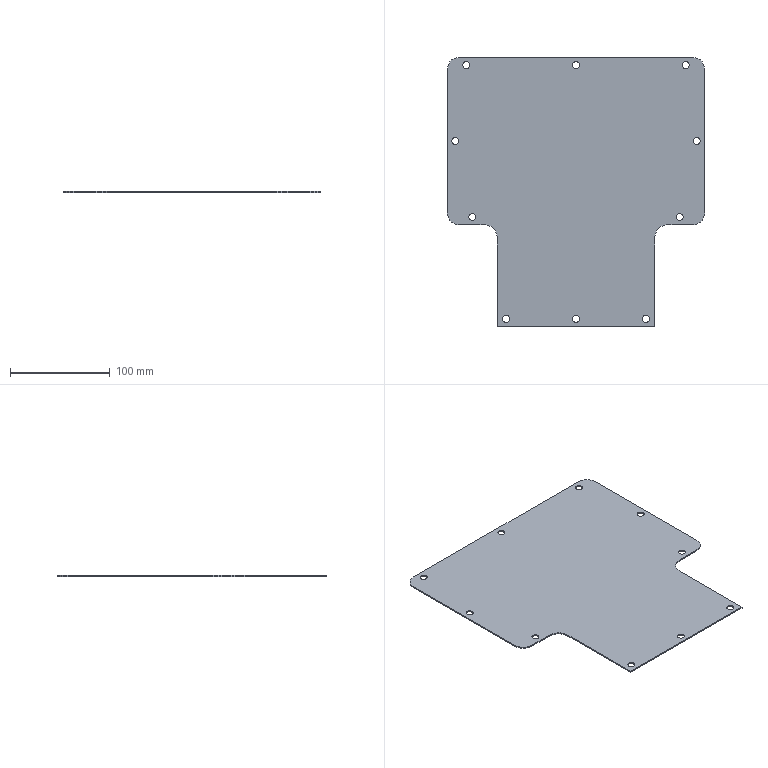Part | SolidWorks | features FlatPattern 1, SMBaseFlange 1, SheetMetal 1 | 1 solid | 36 faces | box 257.6 x 269.6 x 1.2 mm | volume 70578 mm3 | cylinder 26 | plane 10 | commonest cylinder face diameters 7 x20 24 x4 26.4 x2
STEP:
#1=CARTESIAN_POINT('',(14.652,27.28,-1.2));
#2=VERTEX_POINT('',#1);
#3=CARTESIAN_POINT('',(7.652,27.28,-1.2));
#4=VERTEX_POINT('',#3);
#5=CARTESIAN_POINT('',(11.152,27.28,-1.2));
#6=DIRECTION('',(0.,0.,-1.));
#7=DIRECTION('',(-1.,0.,0.));
#8=AXIS2_PLACEMENT_3D('',#5,#6,#7);
#9=CIRCLE('',#8,3.5);
#10=EDGE_CURVE('',#2,#4,#9,.T.);
#11=ORIENTED_EDGE('',*,*,#10,.T.);
#12=CARTESIAN_POINT('',(7.652,27.28,0.));
#13=VERTEX_POINT('',#12);
#14=CARTESIAN_POINT('',(7.652,27.28,-1.2));
#15=DIRECTION('',(0.,0.,1.));
#16=VECTOR('',#15,1000.);
#17=LINE('',#14,#16);
#18=EDGE_CURVE('',#4,#13,#17,.T.);
#19=ORIENTED_EDGE('',*,*,#18,.T.);
#20=CARTESIAN_POINT('',(14.652,27.28,0.));
#21=VERTEX_POINT('',#20);
#22=CARTESIAN_POINT('',(11.152,27.28,0.));
#23=DIRECTION('',(0.,0.,-1.));
#24=DIRECTION('',(-1.,0.,0.));
#25=AXIS2_PLACEMENT_3D('',#22,#23,#24);
#26=CIRCLE('',#25,3.5);
#27=EDGE_CURVE('',#21,#13,#26,.T.);
#28=ORIENTED_EDGE('',*,*,#27,.F.);
#29=CARTESIAN_POINT('',(14.652,27.28,-1.2));
#30=DIRECTION('',(0.,0.,1.));
#31=VECTOR('',#30,1000.);
#32=LINE('',#29,#31);
#33=EDGE_CURVE('',#2,#21,#32,.T.);
#34=ORIENTED_EDGE('',*,*,#33,.F.);
#35=EDGE_LOOP('',(#11,#19,#28,#34));
#36=FACE_OUTER_BOUND('',#35,.T.);
#37=CARTESIAN_POINT('',(11.152,27.28,-1.2));
#38=DIRECTION('',(0.,0.,1.));
#39=DIRECTION('',(1.,0.,0.));
#40=AXIS2_PLACEMENT_3D('',#37,#38,#39);
#41=CYLINDRICAL_SURFACE('',#40,3.5);
#42=ADVANCED_FACE('',(#36),#41,.F.);
#43=CARTESIAN_POINT('',(-2.548,-48.72,-1.2));
#44=VERTEX_POINT('',#43);
#45=CARTESIAN_POINT('',(-9.548,-48.72,-1.2));
#46=VERTEX_POINT('',#45);
#47=CARTESIAN_POINT('',(-6.048,-48.72,-1.2));
#48=DIRECTION('',(0.,0.,-1.));
#49=DIRECTION('',(-1.,0.,0.));
#50=AXIS2_PLACEMENT_3D('',#47,#48,#49);
#51=CIRCLE('',#50,3.5);
#52=EDGE_CURVE('',#44,#46,#51,.T.);
#53=ORIENTED_EDGE('',*,*,#52,.T.);
#54=CARTESIAN_POINT('',(-9.548,-48.72,0.));
#55=VERTEX_POINT('',#54);
#56=CARTESIAN_POINT('',(-9.548,-48.72,-1.2));
#57=DIRECTION('',(0.,0.,1.));
#58=VECTOR('',#57,1000.);
#59=LINE('',#56,#58);
#60=EDGE_CURVE('',#46,#55,#59,.T.);
#61=ORIENTED_EDGE('',*,*,#60,.T.);
#62=CARTESIAN_POINT('',(-2.548,-48.72,0.));
#63=VERTEX_POINT('',#62);
#64=CARTESIAN_POINT('',(-6.048,-48.72,0.));
#65=DIRECTION('',(0.,0.,-1.));
#66=DIRECTION('',(-1.,0.,0.));
#67=AXIS2_PLACEMENT_3D('',#64,#65,#66);
#68=CIRCLE('',#67,3.5);
#69=EDGE_CURVE('',#63,#55,#68,.T.);
#70=ORIENTED_EDGE('',*,*,#69,.F.);
#71=CARTESIAN_POINT('',(-2.548,-48.72,-1.2));
#72=DIRECTION('',(0.,0.,1.));
#73=VECTOR('',#72,1000.);
#74=LINE('',#71,#73);
#75=EDGE_CURVE('',#44,#63,#74,.T.);
#76=ORIENTED_EDGE('',*,*,#75,.F.);
#77=EDGE_LOOP('',(#53,#61,#70,#76));
#78=FACE_OUTER_BOUND('',#77,.T.);
#79=CARTESIAN_POINT('',(-6.048,-48.72,-1.2));
#80=DIRECTION('',(0.,0.,1.));
#81=DIRECTION('',(1.,0.,0.));
#82=AXIS2_PLACEMENT_3D('',#79,#80,#81);
#83=CYLINDRICAL_SURFACE('',#82,3.5);
#84=ADVANCED_FACE('',(#78),#83,.F.);
#85=CARTESIAN_POINT('',(-36.348,-150.72,-1.2));
#86=VERTEX_POINT('',#85);
#87=CARTESIAN_POINT('',(-43.348,-150.72,-1.2));
#88=VERTEX_POINT('',#87);
#89=CARTESIAN_POINT('',(-39.848,-150.72,-1.2));
#90=DIRECTION('',(0.,0.,-1.));
#91=DIRECTION('',(-1.,0.,0.));
#92=AXIS2_PLACEMENT_3D('',#89,#90,#91);
#93=CIRCLE('',#92,3.5);
#94=EDGE_CURVE('',#86,#88,#93,.T.);
#95=ORIENTED_EDGE('',*,*,#94,.T.);
#96=CARTESIAN_POINT('',(-43.348,-150.72,0.));
#97=VERTEX_POINT('',#96);
#98=CARTESIAN_POINT('',(-43.348,-150.72,-1.2));
#99=DIRECTION('',(0.,0.,1.));
#100=VECTOR('',#99,1000.);
#101=LINE('',#98,#100);
#102=EDGE_CURVE('',#88,#97,#101,.T.);
#103=ORIENTED_EDGE('',*,*,#102,.T.);
#104=CARTESIAN_POINT('',(-36.348,-150.72,0.));
#105=VERTEX_POINT('',#104);
#106=CARTESIAN_POINT('',(-39.848,-150.72,0.));
#107=DIRECTION('',(0.,0.,-1.));
#108=DIRECTION('',(-1.,0.,0.));
#109=AXIS2_PLACEMENT_3D('',#106,#107,#108);
#110=CIRCLE('',#109,3.5);
#111=EDGE_CURVE('',#105,#97,#110,.T.);
#112=ORIENTED_EDGE('',*,*,#111,.F.);
#113=CARTESIAN_POINT('',(-36.348,-150.72,-1.2));
#114=DIRECTION('',(0.,0.,1.));
#115=VECTOR('',#114,1000.);
#116=LINE('',#113,#115);
#117=EDGE_CURVE('',#86,#105,#116,.T.);
#118=ORIENTED_EDGE('',*,*,#117,.F.);
#119=EDGE_LOOP('',(#95,#103,#112,#118));
#120=FACE_OUTER_BOUND('',#119,.T.);
#121=CARTESIAN_POINT('',(-39.848,-150.72,-1.2));
#122=DIRECTION('',(0.,0.,1.));
#123=DIRECTION('',(1.,0.,0.));
#124=AXIS2_PLACEMENT_3D('',#121,#122,#123);
#125=CYLINDRICAL_SURFACE('',#124,3.5);
#126=ADVANCED_FACE('',(#120),#125,.F.);
#127=CARTESIAN_POINT('',(-106.348,-150.72,-1.2));
#128=VERTEX_POINT('',#127);
#129=CARTESIAN_POINT('',(-113.348,-150.72,-1.2));
#130=VERTEX_POINT('',#129);
#131=CARTESIAN_POINT('',(-109.848,-150.72,-1.2));
#132=DIRECTION('',(0.,0.,-1.));
#133=DIRECTION('',(-1.,0.,0.));
#134=AXIS2_PLACEMENT_3D('',#131,#132,#133);
#135=CIRCLE('',#134,3.5);
#136=EDGE_CURVE('',#128,#130,#135,.T.);
#137=ORIENTED_EDGE('',*,*,#136,.T.);
#138=CARTESIAN_POINT('',(-113.348,-150.72,0.));
#139=VERTEX_POINT('',#138);
#140=CARTESIAN_POINT('',(-113.348,-150.72,-1.2));
#141=DIRECTION('',(0.,0.,1.));
#142=VECTOR('',#141,1000.);
#143=LINE('',#140,#142);
#144=EDGE_CURVE('',#130,#139,#143,.T.);
#145=ORIENTED_EDGE('',*,*,#144,.T.);
#146=CARTESIAN_POINT('',(-106.348,-150.72,0.));
#147=VERTEX_POINT('',#146);
#148=CARTESIAN_POINT('',(-109.848,-150.72,0.));
#149=DIRECTION('',(0.,0.,-1.));
#150=DIRECTION('',(-1.,0.,0.));
#151=AXIS2_PLACEMENT_3D('',#148,#149,#150);
#152=CIRCLE('',#151,3.5);
#153=EDGE_CURVE('',#147,#139,#152,.T.);
#154=ORIENTED_EDGE('',*,*,#153,.F.);
#155=CARTESIAN_POINT('',(-106.348,-150.72,-1.2));
#156=DIRECTION('',(0.,0.,1.));
#157=VECTOR('',#156,1000.);
#158=LINE('',#155,#157);
#159=EDGE_CURVE('',#128,#147,#158,.T.);
#160=ORIENTED_EDGE('',*,*,#159,.F.);
#161=EDGE_LOOP('',(#137,#145,#154,#160));
#162=FACE_OUTER_BOUND('',#161,.T.);
#163=CARTESIAN_POINT('',(-109.848,-150.72,-1.2));
#164=DIRECTION('',(0.,0.,1.));
#165=DIRECTION('',(1.,0.,0.));
#166=AXIS2_PLACEMENT_3D('',#163,#164,#165);
#167=CYLINDRICAL_SURFACE('',#166,3.5);
#168=ADVANCED_FACE('',(#162),#167,.F.);
#169=CARTESIAN_POINT('',(-176.348,-150.72,-1.2));
#170=VERTEX_POINT('',#169);
#171=CARTESIAN_POINT('',(-183.348,-150.72,-1.2));
#172=VERTEX_POINT('',#171);
#173=CARTESIAN_POINT('',(-179.848,-150.72,-1.2));
#174=DIRECTION('',(0.,0.,-1.));
#175=DIRECTION('',(-1.,0.,0.));
#176=AXIS2_PLACEMENT_3D('',#173,#174,#175);
#177=CIRCLE('',#176,3.5);
#178=EDGE_CURVE('',#170,#172,#177,.T.);
#179=ORIENTED_EDGE('',*,*,#178,.T.);
#180=CARTESIAN_POINT('',(-183.348,-150.72,0.));
#181=VERTEX_POINT('',#180);
#182=CARTESIAN_POINT('',(-183.348,-150.72,-1.2));
#183=DIRECTION('',(0.,0.,1.));
#184=VECTOR('',#183,1000.);
#185=LINE('',#182,#184);
#186=EDGE_CURVE('',#172,#181,#185,.T.);
#187=ORIENTED_EDGE('',*,*,#186,.T.);
#188=CARTESIAN_POINT('',(-176.348,-150.72,0.));
#189=VERTEX_POINT('',#188);
#190=CARTESIAN_POINT('',(-179.848,-150.72,0.));
#191=DIRECTION('',(0.,0.,-1.));
#192=DIRECTION('',(-1.,0.,0.));
#193=AXIS2_PLACEMENT_3D('',#190,#191,#192);
#194=CIRCLE('',#193,3.5);
#195=EDGE_CURVE('',#189,#181,#194,.T.);
#196=ORIENTED_EDGE('',*,*,#195,.F.);
#197=CARTESIAN_POINT('',(-176.348,-150.72,-1.2));
#198=DIRECTION('',(0.,0.,1.));
#199=VECTOR('',#198,1000.);
#200=LINE('',#197,#199);
#201=EDGE_CURVE('',#170,#189,#200,.T.);
#202=ORIENTED_EDGE('',*,*,#201,.F.);
#203=EDGE_LOOP('',(#179,#187,#196,#202));
#204=FACE_OUTER_BOUND('',#203,.T.);
#205=CARTESIAN_POINT('',(-179.848,-150.72,-1.2));
#206=DIRECTION('',(0.,0.,1.));
#207=DIRECTION('',(1.,0.,0.));
#208=AXIS2_PLACEMENT_3D('',#205,#206,#207);
#209=CYLINDRICAL_SURFACE('',#208,3.5);
#210=ADVANCED_FACE('',(#204),#209,.F.);
#211=CARTESIAN_POINT('',(-210.148,-48.72,-1.2));
#212=VERTEX_POINT('',#211);
#213=CARTESIAN_POINT('',(-217.148,-48.72,-1.2));
#214=VERTEX_POINT('',#213);
#215=CARTESIAN_POINT('',(-213.648,-48.72,-1.2));
#216=DIRECTION('',(0.,0.,-1.));
#217=DIRECTION('',(-1.,0.,0.));
#218=AXIS2_PLACEMENT_3D('',#215,#216,#217);
#219=CIRCLE('',#218,3.5);
#220=EDGE_CURVE('',#212,#214,#219,.T.);
#221=ORIENTED_EDGE('',*,*,#220,.T.);
#222=CARTESIAN_POINT('',(-217.148,-48.72,0.));
#223=VERTEX_POINT('',#222);
#224=CARTESIAN_POINT('',(-217.148,-48.72,-1.2));
#225=DIRECTION('',(0.,0.,1.));
#226=VECTOR('',#225,1000.);
#227=LINE('',#224,#226);
#228=EDGE_CURVE('',#214,#223,#227,.T.);
#229=ORIENTED_EDGE('',*,*,#228,.T.);
#230=CARTESIAN_POINT('',(-210.148,-48.72,0.));
#231=VERTEX_POINT('',#230);
#232=CARTESIAN_POINT('',(-213.648,-48.72,0.));
#233=DIRECTION('',(0.,0.,-1.));
#234=DIRECTION('',(-1.,0.,0.));
#235=AXIS2_PLACEMENT_3D('',#232,#233,#234);
#236=CIRCLE('',#235,3.5);
#237=EDGE_CURVE('',#231,#223,#236,.T.);
#238=ORIENTED_EDGE('',*,*,#237,.F.);
#239=CARTESIAN_POINT('',(-210.148,-48.72,-1.2));
#240=DIRECTION('',(0.,0.,1.));
#241=VECTOR('',#240,1000.);
#242=LINE('',#239,#241);
#243=EDGE_CURVE('',#212,#231,#242,.T.);
#244=ORIENTED_EDGE('',*,*,#243,.F.);
#245=EDGE_LOOP('',(#221,#229,#238,#244));
#246=FACE_OUTER_BOUND('',#245,.T.);
#247=CARTESIAN_POINT('',(-213.648,-48.72,-1.2));
#248=DIRECTION('',(0.,0.,1.));
#249=DIRECTION('',(1.,0.,0.));
#250=AXIS2_PLACEMENT_3D('',#247,#248,#249);
#251=CYLINDRICAL_SURFACE('',#250,3.5);
#252=ADVANCED_FACE('',(#246),#251,.F.);
#253=CARTESIAN_POINT('',(-227.348,27.28,-1.2));
#254=VERTEX_POINT('',#253);
#255=CARTESIAN_POINT('',(-234.348,27.28,-1.2));
#256=VERTEX_POINT('',#255);
#257=CARTESIAN_POINT('',(-230.848,27.28,-1.2));
#258=DIRECTION('',(0.,0.,-1.));
#259=DIRECTION('',(-1.,0.,0.));
#260=AXIS2_PLACEMENT_3D('',#257,#258,#259);
#261=CIRCLE('',#260,3.5);
#262=EDGE_CURVE('',#254,#256,#261,.T.);
#263=ORIENTED_EDGE('',*,*,#262,.T.);
#264=CARTESIAN_POINT('',(-234.348,27.28,0.));
#265=VERTEX_POINT('',#264);
#266=CARTESIAN_POINT('',(-234.348,27.28,-1.2));
#267=DIRECTION('',(0.,0.,1.));
#268=VECTOR('',#267,1000.);
#269=LINE('',#266,#268);
#270=EDGE_CURVE('',#256,#265,#269,.T.);
#271=ORIENTED_EDGE('',*,*,#270,.T.);
#272=CARTESIAN_POINT('',(-227.348,27.28,0.));
#273=VERTEX_POINT('',#272);
#274=CARTESIAN_POINT('',(-230.848,27.28,0.));
#275=DIRECTION('',(0.,0.,-1.));
#276=DIRECTION('',(-1.,0.,0.));
#277=AXIS2_PLACEMENT_3D('',#274,#275,#276);
#278=CIRCLE('',#277,3.5);
#279=EDGE_CURVE('',#273,#265,#278,.T.);
#280=ORIENTED_EDGE('',*,*,#279,.F.);
#281=CARTESIAN_POINT('',(-227.348,27.28,-1.2));
#282=DIRECTION('',(0.,0.,1.));
#283=VECTOR('',#282,1000.);
#284=LINE('',#281,#283);
#285=EDGE_CURVE('',#254,#273,#284,.T.);
#286=ORIENTED_EDGE('',*,*,#285,.F.);
#287=EDGE_LOOP('',(#263,#271,#280,#286));
#288=FACE_OUTER_BOUND('',#287,.T.);
#289=CARTESIAN_POINT('',(-230.848,27.28,-1.2));
#290=DIRECTION('',(0.,0.,1.));
#291=DIRECTION('',(1.,0.,0.));
#292=AXIS2_PLACEMENT_3D('',#289,#290,#291);
#293=CYLINDRICAL_SURFACE('',#292,3.5);
#294=ADVANCED_FACE('',(#288),#293,.F.);
#295=CARTESIAN_POINT('',(-216.348,103.28,-1.2));
#296=VERTEX_POINT('',#295);
#297=CARTESIAN_POINT('',(-223.348,103.28,-1.2));
#298=VERTEX_POINT('',#297);
#299=CARTESIAN_POINT('',(-219.848,103.28,-1.2));
#300=DIRECTION('',(0.,0.,-1.));
#301=DIRECTION('',(-1.,0.,0.));
#302=AXIS2_PLACEMENT_3D('',#299,#300,#301);
#303=CIRCLE('',#302,3.5);
#304=EDGE_CURVE('',#296,#298,#303,.T.);
#305=ORIENTED_EDGE('',*,*,#304,.T.);
#306=CARTESIAN_POINT('',(-223.348,103.28,0.));
#307=VERTEX_POINT('',#306);
#308=CARTESIAN_POINT('',(-223.348,103.28,-1.2));
#309=DIRECTION('',(0.,0.,1.));
#310=VECTOR('',#309,1000.);
#311=LINE('',#308,#310);
#312=EDGE_CURVE('',#298,#307,#311,.T.);
#313=ORIENTED_EDGE('',*,*,#312,.T.);
#314=CARTESIAN_POINT('',(-216.348,103.28,0.));
#315=VERTEX_POINT('',#314);
#316=CARTESIAN_POINT('',(-219.848,103.28,0.));
#317=DIRECTION('',(0.,0.,-1.));
#318=DIRECTION('',(-1.,0.,0.));
#319=AXIS2_PLACEMENT_3D('',#316,#317,#318);
#320=CIRCLE('',#319,3.5);
#321=EDGE_CURVE('',#315,#307,#320,.T.);
#322=ORIENTED_EDGE('',*,*,#321,.F.);
#323=CARTESIAN_POINT('',(-216.348,103.28,-1.2));
#324=DIRECTION('',(0.,0.,1.));
#325=VECTOR('',#324,1000.);
#326=LINE('',#323,#325);
#327=EDGE_CURVE('',#296,#315,#326,.T.);
#328=ORIENTED_EDGE('',*,*,#327,.F.);
#329=EDGE_LOOP('',(#305,#313,#322,#328));
#330=FACE_OUTER_BOUND('',#329,.T.);
#331=CARTESIAN_POINT('',(-219.848,103.28,-1.2));
#332=DIRECTION('',(0.,0.,1.));
#333=DIRECTION('',(1.,0.,0.));
#334=AXIS2_PLACEMENT_3D('',#331,#332,#333);
#335=CYLINDRICAL_SURFACE('',#334,3.5);
#336=ADVANCED_FACE('',(#330),#335,.F.);
#337=CARTESIAN_POINT('',(-106.348,103.28,-1.2));
#338=VERTEX_POINT('',#337);
#339=CARTESIAN_POINT('',(-113.348,103.28,-1.2));
#340=VERTEX_POINT('',#339);
#341=CARTESIAN_POINT('',(-109.848,103.28,-1.2));
#342=DIRECTION('',(0.,0.,-1.));
#343=DIRECTION('',(-1.,0.,0.));
#344=AXIS2_PLACEMENT_3D('',#341,#342,#343);
#345=CIRCLE('',#344,3.5);
#346=EDGE_CURVE('',#338,#340,#345,.T.);
#347=ORIENTED_EDGE('',*,*,#346,.T.);
#348=CARTESIAN_POINT('',(-113.348,103.28,0.));
#349=VERTEX_POINT('',#348);
#350=CARTESIAN_POINT('',(-113.348,103.28,-1.2));
#351=DIRECTION('',(0.,0.,1.));
#352=VECTOR('',#351,1000.);
#353=LINE('',#350,#352);
#354=EDGE_CURVE('',#340,#349,#353,.T.);
#355=ORIENTED_EDGE('',*,*,#354,.T.);
#356=CARTESIAN_POINT('',(-106.348,103.28,0.));
#357=VERTEX_POINT('',#356);
#358=CARTESIAN_POINT('',(-109.848,103.28,0.));
#359=DIRECTION('',(0.,0.,-1.));
#360=DIRECTION('',(-1.,0.,0.));
#361=AXIS2_PLACEMENT_3D('',#358,#359,#360);
#362=CIRCLE('',#361,3.5);
#363=EDGE_CURVE('',#357,#349,#362,.T.);
#364=ORIENTED_EDGE('',*,*,#363,.F.);
#365=CARTESIAN_POINT('',(-106.348,103.28,-1.2));
#366=DIRECTION('',(0.,0.,1.));
#367=VECTOR('',#366,1000.);
#368=LINE('',#365,#367);
#369=EDGE_CURVE('',#338,#357,#368,.T.);
#370=ORIENTED_EDGE('',*,*,#369,.F.);
#371=EDGE_LOOP('',(#347,#355,#364,#370));
#372=FACE_OUTER_BOUND('',#371,.T.);
#373=CARTESIAN_POINT('',(-109.848,103.28,-1.2));
#374=DIRECTION('',(0.,0.,1.));
#375=DIRECTION('',(1.,0.,0.));
#376=AXIS2_PLACEMENT_3D('',#373,#374,#375);
#377=CYLINDRICAL_SURFACE('',#376,3.5);
#378=ADVANCED_FACE('',(#372),#377,.F.);
#379=CARTESIAN_POINT('',(3.652,103.28,-1.2));
#380=VERTEX_POINT('',#379);
#381=CARTESIAN_POINT('',(-3.348,103.28,-1.2));
#382=VERTEX_POINT('',#381);
#383=CARTESIAN_POINT('',(0.1516,103.28,-1.2));
#384=DIRECTION('',(0.,0.,-1.));
#385=DIRECTION('',(-1.,0.,0.));
#386=AXIS2_PLACEMENT_3D('',#383,#384,#385);
#387=CIRCLE('',#386,3.5);
#388=EDGE_CURVE('',#380,#382,#387,.T.);
#389=ORIENTED_EDGE('',*,*,#388,.T.);
#390=CARTESIAN_POINT('',(-3.348,103.28,0.));
#391=VERTEX_POINT('',#390);
#392=CARTESIAN_POINT('',(-3.348,103.28,-1.2));
#393=DIRECTION('',(0.,0.,1.));
#394=VECTOR('',#393,1000.);
#395=LINE('',#392,#394);
#396=EDGE_CURVE('',#382,#391,#395,.T.);
#397=ORIENTED_EDGE('',*,*,#396,.T.);
#398=CARTESIAN_POINT('',(3.652,103.28,0.));
#399=VERTEX_POINT('',#398);
#400=CARTESIAN_POINT('',(0.1516,103.28,0.));
#401=DIRECTION('',(0.,0.,-1.));
#402=DIRECTION('',(-1.,0.,0.));
#403=AXIS2_PLACEMENT_3D('',#400,#401,#402);
#404=CIRCLE('',#403,3.5);
#405=EDGE_CURVE('',#399,#391,#404,.T.);
#406=ORIENTED_EDGE('',*,*,#405,.F.);
#407=CARTESIAN_POINT('',(3.652,103.28,-1.2));
#408=DIRECTION('',(0.,0.,1.));
#409=VECTOR('',#408,1000.);
#410=LINE('',#407,#409);
#411=EDGE_CURVE('',#380,#399,#410,.T.);
#412=ORIENTED_EDGE('',*,*,#411,.F.);
#413=EDGE_LOOP('',(#389,#397,#406,#412));
#414=FACE_OUTER_BOUND('',#413,.T.);
#415=CARTESIAN_POINT('',(0.1516,103.28,-1.2));
#416=DIRECTION('',(0.,0.,1.));
#417=DIRECTION('',(1.,0.,0.));
#418=AXIS2_PLACEMENT_3D('',#415,#416,#417);
#419=CYLINDRICAL_SURFACE('',#418,3.5);
#420=ADVANCED_FACE('',(#414),#419,.F.);
#421=ORIENTED_EDGE('',*,*,#52,.F.);
#422=CARTESIAN_POINT('',(-6.048,-48.72,-1.2));
#423=DIRECTION('',(0.,0.,-1.));
#424=DIRECTION('',(-1.,0.,0.));
#425=AXIS2_PLACEMENT_3D('',#422,#423,#424);
#426=CIRCLE('',#425,3.5);
#427=EDGE_CURVE('',#46,#44,#426,.T.);
#428=ORIENTED_EDGE('',*,*,#427,.F.);
#429=EDGE_LOOP('',(#421,#428));
#430=FACE_BOUND('',#429,.T.);
#431=ORIENTED_EDGE('',*,*,#136,.F.);
#432=CARTESIAN_POINT('',(-109.848,-150.72,-1.2));
#433=DIRECTION('',(0.,0.,-1.));
#434=DIRECTION('',(-1.,0.,0.));
#435=AXIS2_PLACEMENT_3D('',#432,#433,#434);
#436=CIRCLE('',#435,3.5);
#437=EDGE_CURVE('',#130,#128,#436,.T.);
#438=ORIENTED_EDGE('',*,*,#437,.F.);
#439=EDGE_LOOP('',(#431,#438));
#440=FACE_BOUND('',#439,.T.);
#441=ORIENTED_EDGE('',*,*,#220,.F.);
#442=CARTESIAN_POINT('',(-213.648,-48.72,-1.2));
#443=DIRECTION('',(0.,0.,-1.));
#444=DIRECTION('',(-1.,0.,0.));
#445=AXIS2_PLACEMENT_3D('',#442,#443,#444);
#446=CIRCLE('',#445,3.5);
#447=EDGE_CURVE('',#214,#212,#446,.T.);
#448=ORIENTED_EDGE('',*,*,#447,.F.);
#449=EDGE_LOOP('',(#441,#448));
#450=FACE_BOUND('',#449,.T.);
#451=ORIENTED_EDGE('',*,*,#304,.F.);
#452=CARTESIAN_POINT('',(-219.848,103.28,-1.2));
#453=DIRECTION('',(0.,0.,-1.));
#454=DIRECTION('',(-1.,0.,0.));
#455=AXIS2_PLACEMENT_3D('',#452,#453,#454);
#456=CIRCLE('',#455,3.5);
#457=EDGE_CURVE('',#298,#296,#456,.T.);
#458=ORIENTED_EDGE('',*,*,#457,.F.);
#459=EDGE_LOOP('',(#451,#458));
#460=FACE_BOUND('',#459,.T.);
#461=ORIENTED_EDGE('',*,*,#388,.F.);
#462=CARTESIAN_POINT('',(0.1516,103.28,-1.2));
#463=DIRECTION('',(0.,0.,-1.));
#464=DIRECTION('',(-1.,0.,0.));
#465=AXIS2_PLACEMENT_3D('',#462,#463,#464);
#466=CIRCLE('',#465,3.5);
#467=EDGE_CURVE('',#382,#380,#466,.T.);
#468=ORIENTED_EDGE('',*,*,#467,.F.);
#469=EDGE_LOOP('',(#461,#468));
#470=FACE_BOUND('',#469,.T.);
#471=CARTESIAN_POINT('',(6.952,111.08,-1.2));
#472=VERTEX_POINT('',#471);
#473=CARTESIAN_POINT('',(18.952,99.08,-1.2));
#474=VERTEX_POINT('',#473);
#475=CARTESIAN_POINT('',(6.952,99.08,-1.2));
#476=DIRECTION('',(0.,0.,-1.));
#477=DIRECTION('',(-1.,0.,0.));
#478=AXIS2_PLACEMENT_3D('',#475,#476,#477);
#479=CIRCLE('',#478,12.);
#480=EDGE_CURVE('',#472,#474,#479,.T.);
#481=ORIENTED_EDGE('',*,*,#480,.T.);
#482=CARTESIAN_POINT('',(18.952,-44.52,-1.2));
#483=VERTEX_POINT('',#482);
#484=CARTESIAN_POINT('',(18.952,99.08,-1.2));
#485=DIRECTION('',(0.,-1.,0.));
#486=VECTOR('',#485,1000.);
#487=LINE('',#484,#486);
#488=EDGE_CURVE('',#474,#483,#487,.T.);
#489=ORIENTED_EDGE('',*,*,#488,.T.);
#490=CARTESIAN_POINT('',(6.952,-56.52,-1.2));
#491=VERTEX_POINT('',#490);
#492=CARTESIAN_POINT('',(6.952,-44.52,-1.2));
#493=DIRECTION('',(0.,0.,-1.));
#494=DIRECTION('',(-1.,0.,0.));
#495=AXIS2_PLACEMENT_3D('',#492,#493,#494);
#496=CIRCLE('',#495,12.);
#497=EDGE_CURVE('',#483,#491,#496,.T.);
#498=ORIENTED_EDGE('',*,*,#497,.T.);
#499=CARTESIAN_POINT('',(-17.848,-56.52,-1.2));
#500=VERTEX_POINT('',#499);
#501=CARTESIAN_POINT('',(6.952,-56.52,-1.2));
#502=DIRECTION('',(-1.,0.,0.));
#503=VECTOR('',#502,1000.);
#504=LINE('',#501,#503);
#505=EDGE_CURVE('',#491,#500,#504,.T.);
#506=ORIENTED_EDGE('',*,*,#505,.T.);
#507=CARTESIAN_POINT('',(-31.048,-69.72,-1.2));
#508=VERTEX_POINT('',#507);
#509=CARTESIAN_POINT('',(-17.848,-69.72,-1.2));
#510=DIRECTION('',(0.,0.,1.));
#511=DIRECTION('',(-1.,0.,0.));
#512=AXIS2_PLACEMENT_3D('',#509,#510,#511);
#513=CIRCLE('',#512,13.2);
#514=EDGE_CURVE('',#500,#508,#513,.T.);
#515=ORIENTED_EDGE('',*,*,#514,.T.);
#516=CARTESIAN_POINT('',(-31.048,-158.52,-1.2));
#517=VERTEX_POINT('',#516);
#518=CARTESIAN_POINT('',(-31.048,-69.72,-1.2));
#519=DIRECTION('',(0.,-1.,0.));
#520=VECTOR('',#519,1000.);
#521=LINE('',#518,#520);
#522=EDGE_CURVE('',#508,#517,#521,.T.);
#523=ORIENTED_EDGE('',*,*,#522,.T.);
#524=CARTESIAN_POINT('',(-188.648,-158.52,-1.2));
#525=VERTEX_POINT('',#524);
#526=CARTESIAN_POINT('',(-31.048,-158.52,-1.2));
#527=DIRECTION('',(-1.,0.,0.));
#528=VECTOR('',#527,1000.);
#529=LINE('',#526,#528);
#530=EDGE_CURVE('',#517,#525,#529,.T.);
#531=ORIENTED_EDGE('',*,*,#530,.T.);
#532=CARTESIAN_POINT('',(-188.648,-69.72,-1.2));
#533=VERTEX_POINT('',#532);
#534=CARTESIAN_POINT('',(-188.648,-158.52,-1.2));
#535=DIRECTION('',(0.,1.,0.));
#536=VECTOR('',#535,1000.);
#537=LINE('',#534,#536);
#538=EDGE_CURVE('',#525,#533,#537,.T.);
#539=ORIENTED_EDGE('',*,*,#538,.T.);
#540=CARTESIAN_POINT('',(-201.848,-56.52,-1.2));
#541=VERTEX_POINT('',#540);
#542=CARTESIAN_POINT('',(-201.848,-69.72,-1.2));
#543=DIRECTION('',(0.,0.,1.));
#544=DIRECTION('',(1.,0.,0.));
#545=AXIS2_PLACEMENT_3D('',#542,#543,#544);
#546=CIRCLE('',#545,13.2);
#547=EDGE_CURVE('',#533,#541,#546,.T.);
#548=ORIENTED_EDGE('',*,*,#547,.T.);
#549=CARTESIAN_POINT('',(-226.648,-56.52,-1.2));
#550=VERTEX_POINT('',#549);
#551=CARTESIAN_POINT('',(-201.848,-56.52,-1.2));
#552=DIRECTION('',(-1.,0.,0.));
#553=VECTOR('',#552,1000.);
#554=LINE('',#551,#553);
#555=EDGE_CURVE('',#541,#550,#554,.T.);
#556=ORIENTED_EDGE('',*,*,#555,.T.);
#557=CARTESIAN_POINT('',(-238.648,-44.52,-1.2));
#558=VERTEX_POINT('',#557);
#559=CARTESIAN_POINT('',(-226.648,-44.52,-1.2));
#560=DIRECTION('',(0.,0.,-1.));
#561=DIRECTION('',(-1.,0.,0.));
#562=AXIS2_PLACEMENT_3D('',#559,#560,#561);
#563=CIRCLE('',#562,12.);
#564=EDGE_CURVE('',#550,#558,#563,.T.);
#565=ORIENTED_EDGE('',*,*,#564,.T.);
#566=CARTESIAN_POINT('',(-238.648,99.08,-1.2));
#567=VERTEX_POINT('',#566);
#568=CARTESIAN_POINT('',(-238.648,-44.52,-1.2));
#569=DIRECTION('',(0.,1.,0.));
#570=VECTOR('',#569,1000.);
#571=LINE('',#568,#570);
#572=EDGE_CURVE('',#558,#567,#571,.T.);
#573=ORIENTED_EDGE('',*,*,#572,.T.);
#574=CARTESIAN_POINT('',(-226.648,111.08,-1.2));
#575=VERTEX_POINT('',#574);
#576=CARTESIAN_POINT('',(-226.648,99.08,-1.2));
#577=DIRECTION('',(0.,0.,-1.));
#578=DIRECTION('',(-1.,0.,0.));
#579=AXIS2_PLACEMENT_3D('',#576,#577,#578);
#580=CIRCLE('',#579,12.);
#581=EDGE_CURVE('',#567,#575,#580,.T.);
#582=ORIENTED_EDGE('',*,*,#581,.T.);
#583=CARTESIAN_POINT('',(-226.648,111.08,-1.2));
#584=DIRECTION('',(1.,0.,0.));
#585=VECTOR('',#584,1000.);
#586=LINE('',#583,#585);
#587=EDGE_CURVE('',#575,#472,#586,.T.);
#588=ORIENTED_EDGE('',*,*,#587,.T.);
#589=EDGE_LOOP('',(#481,#489,#498,#506,#515,#523,#531,#539,#548,#556,#565,#573,#582,#588));
#590=FACE_OUTER_BOUND('',#589,.T.);
#591=ORIENTED_EDGE('',*,*,#346,.F.);
#592=CARTESIAN_POINT('',(-109.848,103.28,-1.2));
#593=DIRECTION('',(0.,0.,-1.));
#594=DIRECTION('',(-1.,0.,0.));
#595=AXIS2_PLACEMENT_3D('',#592,#593,#594);
#596=CIRCLE('',#595,3.5);
#597=EDGE_CURVE('',#340,#338,#596,.T.);
#598=ORIENTED_EDGE('',*,*,#597,.F.);
#599=EDGE_LOOP('',(#591,#598));
#600=FACE_BOUND('',#599,.T.);
#601=ORIENTED_EDGE('',*,*,#262,.F.);
#602=CARTESIAN_POINT('',(-230.848,27.28,-1.2));
#603=DIRECTION('',(0.,0.,-1.));
#604=DIRECTION('',(-1.,0.,0.));
#605=AXIS2_PLACEMENT_3D('',#602,#603,#604);
#606=CIRCLE('',#605,3.5);
#607=EDGE_CURVE('',#256,#254,#606,.T.);
#608=ORIENTED_EDGE('',*,*,#607,.F.);
#609=EDGE_LOOP('',(#601,#608));
#610=FACE_BOUND('',#609,.T.);
#611=ORIENTED_EDGE('',*,*,#178,.F.);
#612=CARTESIAN_POINT('',(-179.848,-150.72,-1.2));
#613=DIRECTION('',(0.,0.,-1.));
#614=DIRECTION('',(-1.,0.,0.));
#615=AXIS2_PLACEMENT_3D('',#612,#613,#614);
#616=CIRCLE('',#615,3.5);
#617=EDGE_CURVE('',#172,#170,#616,.T.);
#618=ORIENTED_EDGE('',*,*,#617,.F.);
#619=EDGE_LOOP('',(#611,#618));
#620=FACE_BOUND('',#619,.T.);
#621=ORIENTED_EDGE('',*,*,#94,.F.);
#622=CARTESIAN_POINT('',(-39.848,-150.72,-1.2));
#623=DIRECTION('',(0.,0.,-1.));
#624=DIRECTION('',(-1.,0.,0.));
#625=AXIS2_PLACEMENT_3D('',#622,#623,#624);
#626=CIRCLE('',#625,3.5);
#627=EDGE_CURVE('',#88,#86,#626,.T.);
#628=ORIENTED_EDGE('',*,*,#627,.F.);
#629=EDGE_LOOP('',(#621,#628));
#630=FACE_BOUND('',#629,.T.);
#631=ORIENTED_EDGE('',*,*,#10,.F.);
#632=CARTESIAN_POINT('',(11.152,27.28,-1.2));
#633=DIRECTION('',(0.,0.,-1.));
#634=DIRECTION('',(-1.,0.,0.));
#635=AXIS2_PLACEMENT_3D('',#632,#633,#634);
#636=CIRCLE('',#635,3.5);
#637=EDGE_CURVE('',#4,#2,#636,.T.);
#638=ORIENTED_EDGE('',*,*,#637,.F.);
#639=EDGE_LOOP('',(#631,#638));
#640=FACE_BOUND('',#639,.T.);
#641=CARTESIAN_POINT('',(6.952,99.08,-1.2));
#642=DIRECTION('',(0.,0.,-1.));
#643=DIRECTION('',(-1.,0.,0.));
#644=AXIS2_PLACEMENT_3D('',#641,#642,#643);
#645=PLANE('',#644);
#646=ADVANCED_FACE('',(#430,#440,#450,#460,#470,#590,#600,#610,#620,#630,#640),#645,.T.);
#647=CARTESIAN_POINT('',(6.952,111.08,0.));
#648=VERTEX_POINT('',#647);
#649=CARTESIAN_POINT('',(18.952,99.08,0.));
#650=VERTEX_POINT('',#649);
#651=CARTESIAN_POINT('',(6.952,99.08,0.));
#652=DIRECTION('',(0.,0.,-1.));
#653=DIRECTION('',(-1.,0.,0.));
#654=AXIS2_PLACEMENT_3D('',#651,#652,#653);
#655=CIRCLE('',#654,12.);
#656=EDGE_CURVE('',#648,#650,#655,.T.);
#657=ORIENTED_EDGE('',*,*,#656,.F.);
#658=CARTESIAN_POINT('',(-226.648,111.08,0.));
#659=VERTEX_POINT('',#658);
#660=CARTESIAN_POINT('',(-226.648,111.08,0.));
#661=DIRECTION('',(1.,0.,0.));
#662=VECTOR('',#661,1000.);
#663=LINE('',#660,#662);
#664=EDGE_CURVE('',#659,#648,#663,.T.);
#665=ORIENTED_EDGE('',*,*,#664,.F.);
#666=CARTESIAN_POINT('',(-238.648,99.08,0.));
#667=VERTEX_POINT('',#666);
#668=CARTESIAN_POINT('',(-226.648,99.08,0.));
#669=DIRECTION('',(0.,0.,-1.));
#670=DIRECTION('',(-1.,0.,0.));
#671=AXIS2_PLACEMENT_3D('',#668,#669,#670);
#672=CIRCLE('',#671,12.);
#673=EDGE_CURVE('',#667,#659,#672,.T.);
#674=ORIENTED_EDGE('',*,*,#673,.F.);
#675=CARTESIAN_POINT('',(-238.648,-44.52,0.));
#676=VERTEX_POINT('',#675);
#677=CARTESIAN_POINT('',(-238.648,-44.52,0.));
#678=DIRECTION('',(0.,1.,0.));
#679=VECTOR('',#678,1000.);
#680=LINE('',#677,#679);
#681=EDGE_CURVE('',#676,#667,#680,.T.);
#682=ORIENTED_EDGE('',*,*,#681,.F.);
#683=CARTESIAN_POINT('',(-226.648,-56.52,0.));
#684=VERTEX_POINT('',#683);
#685=CARTESIAN_POINT('',(-226.648,-44.52,0.));
#686=DIRECTION('',(0.,0.,-1.));
#687=DIRECTION('',(-1.,0.,0.));
#688=AXIS2_PLACEMENT_3D('',#685,#686,#687);
#689=CIRCLE('',#688,12.);
#690=EDGE_CURVE('',#684,#676,#689,.T.);
#691=ORIENTED_EDGE('',*,*,#690,.F.);
#692=CARTESIAN_POINT('',(-201.848,-56.52,0.));
#693=VERTEX_POINT('',#692);
#694=CARTESIAN_POINT('',(-201.848,-56.52,0.));
#695=DIRECTION('',(-1.,0.,0.));
#696=VECTOR('',#695,1000.);
#697=LINE('',#694,#696);
#698=EDGE_CURVE('',#693,#684,#697,.T.);
#699=ORIENTED_EDGE('',*,*,#698,.F.);
#700=CARTESIAN_POINT('',(-188.648,-69.72,0.));
#701=VERTEX_POINT('',#700);
#702=CARTESIAN_POINT('',(-201.848,-69.72,0.));
#703=DIRECTION('',(0.,0.,1.));
#704=DIRECTION('',(1.,0.,0.));
#705=AXIS2_PLACEMENT_3D('',#702,#703,#704);
#706=CIRCLE('',#705,13.2);
#707=EDGE_CURVE('',#701,#693,#706,.T.);
#708=ORIENTED_EDGE('',*,*,#707,.F.);
#709=CARTESIAN_POINT('',(-188.648,-158.52,0.));
#710=VERTEX_POINT('',#709);
#711=CARTESIAN_POINT('',(-188.648,-158.52,0.));
#712=DIRECTION('',(0.,1.,0.));
#713=VECTOR('',#712,1000.);
#714=LINE('',#711,#713);
#715=EDGE_CURVE('',#710,#701,#714,.T.);
#716=ORIENTED_EDGE('',*,*,#715,.F.);
#717=CARTESIAN_POINT('',(-31.048,-158.52,0.));
#718=VERTEX_POINT('',#717);
#719=CARTESIAN_POINT('',(-31.048,-158.52,0.));
#720=DIRECTION('',(-1.,0.,0.));
#721=VECTOR('',#720,1000.);
#722=LINE('',#719,#721);
#723=EDGE_CURVE('',#718,#710,#722,.T.);
#724=ORIENTED_EDGE('',*,*,#723,.F.);
#725=CARTESIAN_POINT('',(-31.048,-69.72,0.));
#726=VERTEX_POINT('',#725);
#727=CARTESIAN_POINT('',(-31.048,-69.72,0.));
#728=DIRECTION('',(0.,-1.,0.));
#729=VECTOR('',#728,1000.);
#730=LINE('',#727,#729);
#731=EDGE_CURVE('',#726,#718,#730,.T.);
#732=ORIENTED_EDGE('',*,*,#731,.F.);
#733=CARTESIAN_POINT('',(-17.848,-56.52,0.));
#734=VERTEX_POINT('',#733);
#735=CARTESIAN_POINT('',(-17.848,-69.72,0.));
#736=DIRECTION('',(0.,0.,1.));
#737=DIRECTION('',(-1.,0.,0.));
#738=AXIS2_PLACEMENT_3D('',#735,#736,#737);
#739=CIRCLE('',#738,13.2);
#740=EDGE_CURVE('',#734,#726,#739,.T.);
#741=ORIENTED_EDGE('',*,*,#740,.F.);
#742=CARTESIAN_POINT('',(6.952,-56.52,0.));
#743=VERTEX_POINT('',#742);
#744=CARTESIAN_POINT('',(6.952,-56.52,0.));
#745=DIRECTION('',(-1.,0.,0.));
#746=VECTOR('',#745,1000.);
#747=LINE('',#744,#746);
#748=EDGE_CURVE('',#743,#734,#747,.T.);
#749=ORIENTED_EDGE('',*,*,#748,.F.);
#750=CARTESIAN_POINT('',(18.952,-44.52,0.));
#751=VERTEX_POINT('',#750);
#752=CARTESIAN_POINT('',(6.952,-44.52,0.));
#753=DIRECTION('',(0.,0.,-1.));
#754=DIRECTION('',(-1.,0.,0.));
#755=AXIS2_PLACEMENT_3D('',#752,#753,#754);
#756=CIRCLE('',#755,12.);
#757=EDGE_CURVE('',#751,#743,#756,.T.);
#758=ORIENTED_EDGE('',*,*,#757,.F.);
#759=CARTESIAN_POINT('',(18.952,99.08,0.));
#760=DIRECTION('',(0.,-1.,0.));
#761=VECTOR('',#760,1000.);
#762=LINE('',#759,#761);
#763=EDGE_CURVE('',#650,#751,#762,.T.);
#764=ORIENTED_EDGE('',*,*,#763,.F.);
#765=EDGE_LOOP('',(#657,#665,#674,#682,#691,#699,#708,#716,#724,#732,#741,#749,#758,#764));
#766=FACE_OUTER_BOUND('',#765,.T.);
#767=ORIENTED_EDGE('',*,*,#405,.T.);
#768=CARTESIAN_POINT('',(0.1516,103.28,0.));
#769=DIRECTION('',(0.,0.,-1.));
#770=DIRECTION('',(-1.,0.,0.));
#771=AXIS2_PLACEMENT_3D('',#768,#769,#770);
#772=CIRCLE('',#771,3.5);
#773=EDGE_CURVE('',#391,#399,#772,.T.);
#774=ORIENTED_EDGE('',*,*,#773,.T.);
#775=EDGE_LOOP('',(#767,#774));
#776=FACE_BOUND('',#775,.T.);
#777=ORIENTED_EDGE('',*,*,#363,.T.);
#778=CARTESIAN_POINT('',(-109.848,103.28,0.));
#779=DIRECTION('',(0.,0.,-1.));
#780=DIRECTION('',(-1.,0.,0.));
#781=AXIS2_PLACEMENT_3D('',#778,#779,#780);
#782=CIRCLE('',#781,3.5);
#783=EDGE_CURVE('',#349,#357,#782,.T.);
#784=ORIENTED_EDGE('',*,*,#783,.T.);
#785=EDGE_LOOP('',(#777,#784));
#786=FACE_BOUND('',#785,.T.);
#787=ORIENTED_EDGE('',*,*,#321,.T.);
#788=CARTESIAN_POINT('',(-219.848,103.28,0.));
#789=DIRECTION('',(0.,0.,-1.));
#790=DIRECTION('',(-1.,0.,0.));
#791=AXIS2_PLACEMENT_3D('',#788,#789,#790);
#792=CIRCLE('',#791,3.5);
#793=EDGE_CURVE('',#307,#315,#792,.T.);
#794=ORIENTED_EDGE('',*,*,#793,.T.);
#795=EDGE_LOOP('',(#787,#794));
#796=FACE_BOUND('',#795,.T.);
#797=ORIENTED_EDGE('',*,*,#279,.T.);
#798=CARTESIAN_POINT('',(-230.848,27.28,0.));
#799=DIRECTION('',(0.,0.,-1.));
#800=DIRECTION('',(-1.,0.,0.));
#801=AXIS2_PLACEMENT_3D('',#798,#799,#800);
#802=CIRCLE('',#801,3.5);
#803=EDGE_CURVE('',#265,#273,#802,.T.);
#804=ORIENTED_EDGE('',*,*,#803,.T.);
#805=EDGE_LOOP('',(#797,#804));
#806=FACE_BOUND('',#805,.T.);
#807=ORIENTED_EDGE('',*,*,#237,.T.);
#808=CARTESIAN_POINT('',(-213.648,-48.72,0.));
#809=DIRECTION('',(0.,0.,-1.));
#810=DIRECTION('',(-1.,0.,0.));
#811=AXIS2_PLACEMENT_3D('',#808,#809,#810);
#812=CIRCLE('',#811,3.5);
#813=EDGE_CURVE('',#223,#231,#812,.T.);
#814=ORIENTED_EDGE('',*,*,#813,.T.);
#815=EDGE_LOOP('',(#807,#814));
#816=FACE_BOUND('',#815,.T.);
#817=ORIENTED_EDGE('',*,*,#195,.T.);
#818=CARTESIAN_POINT('',(-179.848,-150.72,0.));
#819=DIRECTION('',(0.,0.,-1.));
#820=DIRECTION('',(-1.,0.,0.));
#821=AXIS2_PLACEMENT_3D('',#818,#819,#820);
#822=CIRCLE('',#821,3.5);
#823=EDGE_CURVE('',#181,#189,#822,.T.);
#824=ORIENTED_EDGE('',*,*,#823,.T.);
#825=EDGE_LOOP('',(#817,#824));
#826=FACE_BOUND('',#825,.T.);
#827=ORIENTED_EDGE('',*,*,#153,.T.);
#828=CARTESIAN_POINT('',(-109.848,-150.72,0.));
#829=DIRECTION('',(0.,0.,-1.));
#830=DIRECTION('',(-1.,0.,0.));
#831=AXIS2_PLACEMENT_3D('',#828,#829,#830);
#832=CIRCLE('',#831,3.5);
#833=EDGE_CURVE('',#139,#147,#832,.T.);
#834=ORIENTED_EDGE('',*,*,#833,.T.);
#835=EDGE_LOOP('',(#827,#834));
#836=FACE_BOUND('',#835,.T.);
#837=ORIENTED_EDGE('',*,*,#111,.T.);
#838=CARTESIAN_POINT('',(-39.848,-150.72,0.));
#839=DIRECTION('',(0.,0.,-1.));
#840=DIRECTION('',(-1.,0.,0.));
#841=AXIS2_PLACEMENT_3D('',#838,#839,#840);
#842=CIRCLE('',#841,3.5);
#843=EDGE_CURVE('',#97,#105,#842,.T.);
#844=ORIENTED_EDGE('',*,*,#843,.T.);
#845=EDGE_LOOP('',(#837,#844));
#846=FACE_BOUND('',#845,.T.);
#847=ORIENTED_EDGE('',*,*,#69,.T.);
#848=CARTESIAN_POINT('',(-6.048,-48.72,0.));
#849=DIRECTION('',(0.,0.,-1.));
#850=DIRECTION('',(-1.,0.,0.));
#851=AXIS2_PLACEMENT_3D('',#848,#849,#850);
#852=CIRCLE('',#851,3.5);
#853=EDGE_CURVE('',#55,#63,#852,.T.);
#854=ORIENTED_EDGE('',*,*,#853,.T.);
#855=EDGE_LOOP('',(#847,#854));
#856=FACE_BOUND('',#855,.T.);
#857=ORIENTED_EDGE('',*,*,#27,.T.);
#858=CARTESIAN_POINT('',(11.152,27.28,0.));
#859=DIRECTION('',(0.,0.,-1.));
#860=DIRECTION('',(-1.,0.,0.));
#861=AXIS2_PLACEMENT_3D('',#858,#859,#860);
#862=CIRCLE('',#861,3.5);
#863=EDGE_CURVE('',#13,#21,#862,.T.);
#864=ORIENTED_EDGE('',*,*,#863,.T.);
#865=EDGE_LOOP('',(#857,#864));
#866=FACE_BOUND('',#865,.T.);
#867=CARTESIAN_POINT('',(6.952,99.08,0.));
#868=DIRECTION('',(0.,0.,-1.));
#869=DIRECTION('',(-1.,0.,0.));
#870=AXIS2_PLACEMENT_3D('',#867,#868,#869);
#871=PLANE('',#870);
#872=ADVANCED_FACE('',(#766,#776,#786,#796,#806,#816,#826,#836,#846,#856,#866),#871,.F.);
#873=ORIENTED_EDGE('',*,*,#656,.T.);
#874=CARTESIAN_POINT('',(18.952,99.08,-1.2));
#875=DIRECTION('',(0.,0.,1.));
#876=VECTOR('',#875,1000.);
#877=LINE('',#874,#876);
#878=EDGE_CURVE('',#474,#650,#877,.T.);
#879=ORIENTED_EDGE('',*,*,#878,.F.);
#880=ORIENTED_EDGE('',*,*,#480,.F.);
#881=CARTESIAN_POINT('',(6.952,111.08,-1.2));
#882=DIRECTION('',(0.,0.,1.));
#883=VECTOR('',#882,1000.);
#884=LINE('',#881,#883);
#885=EDGE_CURVE('',#472,#648,#884,.T.);
#886=ORIENTED_EDGE('',*,*,#885,.T.);
#887=EDGE_LOOP('',(#873,#879,#880,#886));
#888=FACE_OUTER_BOUND('',#887,.T.);
#889=CARTESIAN_POINT('',(6.952,99.08,-1.2));
#890=DIRECTION('',(0.,0.,1.));
#891=DIRECTION('',(1.,0.,0.));
#892=AXIS2_PLACEMENT_3D('',#889,#890,#891);
#893=CYLINDRICAL_SURFACE('',#892,12.);
#894=ADVANCED_FACE('',(#888),#893,.T.);
#895=ORIENTED_EDGE('',*,*,#763,.T.);
#896=CARTESIAN_POINT('',(18.952,-44.52,-1.2));
#897=DIRECTION('',(0.,0.,1.));
#898=VECTOR('',#897,1000.);
#899=LINE('',#896,#898);
#900=EDGE_CURVE('',#483,#751,#899,.T.);
#901=ORIENTED_EDGE('',*,*,#900,.F.);
#902=ORIENTED_EDGE('',*,*,#488,.F.);
#903=ORIENTED_EDGE('',*,*,#878,.T.);
#904=EDGE_LOOP('',(#895,#901,#902,#903));
#905=FACE_OUTER_BOUND('',#904,.T.);
#906=CARTESIAN_POINT('',(18.952,99.08,-1.2));
#907=DIRECTION('',(-1.,0.,0.));
#908=DIRECTION('',(0.,-1.,0.));
#909=AXIS2_PLACEMENT_3D('',#906,#907,#908);
#910=PLANE('',#909);
#911=ADVANCED_FACE('',(#905),#910,.F.);
#912=ORIENTED_EDGE('',*,*,#757,.T.);
#913=CARTESIAN_POINT('',(6.952,-56.52,-1.2));
#914=DIRECTION('',(0.,0.,1.));
#915=VECTOR('',#914,1000.);
#916=LINE('',#913,#915);
#917=EDGE_CURVE('',#491,#743,#916,.T.);
#918=ORIENTED_EDGE('',*,*,#917,.F.);
#919=ORIENTED_EDGE('',*,*,#497,.F.);
#920=ORIENTED_EDGE('',*,*,#900,.T.);
#921=EDGE_LOOP('',(#912,#918,#919,#920));
#922=FACE_OUTER_BOUND('',#921,.T.);
#923=CARTESIAN_POINT('',(6.952,-44.52,-1.2));
#924=DIRECTION('',(0.,0.,1.));
#925=DIRECTION('',(1.,0.,0.));
#926=AXIS2_PLACEMENT_3D('',#923,#924,#925);
#927=CYLINDRICAL_SURFACE('',#926,12.);
#928=ADVANCED_FACE('',(#922),#927,.T.);
#929=ORIENTED_EDGE('',*,*,#748,.T.);
#930=CARTESIAN_POINT('',(-17.848,-56.52,-1.2));
#931=DIRECTION('',(0.,0.,1.));
#932=VECTOR('',#931,1000.);
#933=LINE('',#930,#932);
#934=EDGE_CURVE('',#500,#734,#933,.T.);
#935=ORIENTED_EDGE('',*,*,#934,.F.);
#936=ORIENTED_EDGE('',*,*,#505,.F.);
#937=ORIENTED_EDGE('',*,*,#917,.T.);
#938=EDGE_LOOP('',(#929,#935,#936,#937));
#939=FACE_OUTER_BOUND('',#938,.T.);
#940=CARTESIAN_POINT('',(6.952,-56.52,-1.2));
#941=DIRECTION('',(0.,1.,0.));
#942=DIRECTION('',(0.,0.,1.));
#943=AXIS2_PLACEMENT_3D('',#940,#941,#942);
#944=PLANE('',#943);
#945=ADVANCED_FACE('',(#939),#944,.F.);
#946=ORIENTED_EDGE('',*,*,#740,.T.);
#947=CARTESIAN_POINT('',(-31.048,-69.72,-1.2));
#948=DIRECTION('',(0.,0.,1.));
#949=VECTOR('',#948,1000.);
#950=LINE('',#947,#949);
#951=EDGE_CURVE('',#508,#726,#950,.T.);
#952=ORIENTED_EDGE('',*,*,#951,.F.);
#953=ORIENTED_EDGE('',*,*,#514,.F.);
#954=ORIENTED_EDGE('',*,*,#934,.T.);
#955=EDGE_LOOP('',(#946,#952,#953,#954));
#956=FACE_OUTER_BOUND('',#955,.T.);
#957=CARTESIAN_POINT('',(-17.848,-69.72,-1.2));
#958=DIRECTION('',(0.,0.,1.));
#959=DIRECTION('',(1.,0.,0.));
#960=AXIS2_PLACEMENT_3D('',#957,#958,#959);
#961=CYLINDRICAL_SURFACE('',#960,13.2);
#962=ADVANCED_FACE('',(#956),#961,.F.);
#963=ORIENTED_EDGE('',*,*,#731,.T.);
#964=CARTESIAN_POINT('',(-31.048,-158.52,-1.2));
#965=DIRECTION('',(0.,0.,1.));
#966=VECTOR('',#965,1000.);
#967=LINE('',#964,#966);
#968=EDGE_CURVE('',#517,#718,#967,.T.);
#969=ORIENTED_EDGE('',*,*,#968,.F.);
#970=ORIENTED_EDGE('',*,*,#522,.F.);
#971=ORIENTED_EDGE('',*,*,#951,.T.);
#972=EDGE_LOOP('',(#963,#969,#970,#971));
#973=FACE_OUTER_BOUND('',#972,.T.);
#974=CARTESIAN_POINT('',(-31.048,-69.72,-1.2));
#975=DIRECTION('',(-1.,0.,0.));
#976=DIRECTION('',(0.,-1.,0.));
#977=AXIS2_PLACEMENT_3D('',#974,#975,#976);
#978=PLANE('',#977);
#979=ADVANCED_FACE('',(#973),#978,.F.);
#980=ORIENTED_EDGE('',*,*,#723,.T.);
#981=CARTESIAN_POINT('',(-188.648,-158.52,-1.2));
#982=DIRECTION('',(0.,0.,1.));
#983=VECTOR('',#982,1000.);
#984=LINE('',#981,#983);
#985=EDGE_CURVE('',#525,#710,#984,.T.);
#986=ORIENTED_EDGE('',*,*,#985,.F.);
#987=ORIENTED_EDGE('',*,*,#530,.F.);
#988=ORIENTED_EDGE('',*,*,#968,.T.);
#989=EDGE_LOOP('',(#980,#986,#987,#988));
#990=FACE_OUTER_BOUND('',#989,.T.);
#991=CARTESIAN_POINT('',(-31.048,-158.52,-1.2));
#992=DIRECTION('',(0.,1.,0.));
#993=DIRECTION('',(0.,0.,1.));
#994=AXIS2_PLACEMENT_3D('',#991,#992,#993);
#995=PLANE('',#994);
#996=ADVANCED_FACE('',(#990),#995,.F.);
#997=ORIENTED_EDGE('',*,*,#715,.T.);
#998=CARTESIAN_POINT('',(-188.648,-69.72,-1.2));
#999=DIRECTION('',(0.,0.,1.));
#1000=VECTOR('',#999,1000.);
#1001=LINE('',#998,#1000);
#1002=EDGE_CURVE('',#533,#701,#1001,.T.);
#1003=ORIENTED_EDGE('',*,*,#1002,.F.);
#1004=ORIENTED_EDGE('',*,*,#538,.F.);
#1005=ORIENTED_EDGE('',*,*,#985,.T.);
#1006=EDGE_LOOP('',(#997,#1003,#1004,#1005));
#1007=FACE_OUTER_BOUND('',#1006,.T.);
#1008=CARTESIAN_POINT('',(-188.648,-158.52,-1.2));
#1009=DIRECTION('',(1.,0.,0.));
#1010=DIRECTION('',(0.,0.,-1.));
#1011=AXIS2_PLACEMENT_3D('',#1008,#1009,#1010);
#1012=PLANE('',#1011);
#1013=ADVANCED_FACE('',(#1007),#1012,.F.);
#1014=ORIENTED_EDGE('',*,*,#707,.T.);
#1015=CARTESIAN_POINT('',(-201.848,-56.52,-1.2));
#1016=DIRECTION('',(0.,0.,1.));
#1017=VECTOR('',#1016,1000.);
#1018=LINE('',#1015,#1017);
#1019=EDGE_CURVE('',#541,#693,#1018,.T.);
#1020=ORIENTED_EDGE('',*,*,#1019,.F.);
#1021=ORIENTED_EDGE('',*,*,#547,.F.);
#1022=ORIENTED_EDGE('',*,*,#1002,.T.);
#1023=EDGE_LOOP('',(#1014,#1020,#1021,#1022));
#1024=FACE_OUTER_BOUND('',#1023,.T.);
#1025=CARTESIAN_POINT('',(-201.848,-69.72,-1.2));
#1026=DIRECTION('',(0.,0.,1.));
#1027=DIRECTION('',(1.,0.,0.));
#1028=AXIS2_PLACEMENT_3D('',#1025,#1026,#1027);
#1029=CYLINDRICAL_SURFACE('',#1028,13.2);
#1030=ADVANCED_FACE('',(#1024),#1029,.F.);
#1031=ORIENTED_EDGE('',*,*,#698,.T.);
#1032=CARTESIAN_POINT('',(-226.648,-56.52,-1.2));
#1033=DIRECTION('',(0.,0.,1.));
#1034=VECTOR('',#1033,1000.);
#1035=LINE('',#1032,#1034);
#1036=EDGE_CURVE('',#550,#684,#1035,.T.);
#1037=ORIENTED_EDGE('',*,*,#1036,.F.);
#1038=ORIENTED_EDGE('',*,*,#555,.F.);
#1039=ORIENTED_EDGE('',*,*,#1019,.T.);
#1040=EDGE_LOOP('',(#1031,#1037,#1038,#1039));
#1041=FACE_OUTER_BOUND('',#1040,.T.);
#1042=CARTESIAN_POINT('',(-201.848,-56.52,-1.2));
#1043=DIRECTION('',(0.,1.,0.));
#1044=DIRECTION('',(-1.,0.,0.));
#1045=AXIS2_PLACEMENT_3D('',#1042,#1043,#1044);
#1046=PLANE('',#1045);
#1047=ADVANCED_FACE('',(#1041),#1046,.F.);
#1048=ORIENTED_EDGE('',*,*,#690,.T.);
#1049=CARTESIAN_POINT('',(-238.648,-44.52,-1.2));
#1050=DIRECTION('',(0.,0.,1.));
#1051=VECTOR('',#1050,1000.);
#1052=LINE('',#1049,#1051);
#1053=EDGE_CURVE('',#558,#676,#1052,.T.);
#1054=ORIENTED_EDGE('',*,*,#1053,.F.);
#1055=ORIENTED_EDGE('',*,*,#564,.F.);
#1056=ORIENTED_EDGE('',*,*,#1036,.T.);
#1057=EDGE_LOOP('',(#1048,#1054,#1055,#1056));
#1058=FACE_OUTER_BOUND('',#1057,.T.);
#1059=CARTESIAN_POINT('',(-226.648,-44.52,-1.2));
#1060=DIRECTION('',(0.,0.,1.));
#1061=DIRECTION('',(1.,0.,0.));
#1062=AXIS2_PLACEMENT_3D('',#1059,#1060,#1061);
#1063=CYLINDRICAL_SURFACE('',#1062,12.);
#1064=ADVANCED_FACE('',(#1058),#1063,.T.);
#1065=ORIENTED_EDGE('',*,*,#681,.T.);
#1066=CARTESIAN_POINT('',(-238.648,99.08,-1.2));
#1067=DIRECTION('',(0.,0.,1.));
#1068=VECTOR('',#1067,1000.);
#1069=LINE('',#1066,#1068);
#1070=EDGE_CURVE('',#567,#667,#1069,.T.);
#1071=ORIENTED_EDGE('',*,*,#1070,.F.);
#1072=ORIENTED_EDGE('',*,*,#572,.F.);
#1073=ORIENTED_EDGE('',*,*,#1053,.T.);
#1074=EDGE_LOOP('',(#1065,#1071,#1072,#1073));
#1075=FACE_OUTER_BOUND('',#1074,.T.);
#1076=CARTESIAN_POINT('',(-238.648,-44.52,-1.2));
#1077=DIRECTION('',(1.,0.,0.));
#1078=DIRECTION('',(0.,1.,0.));
#1079=AXIS2_PLACEMENT_3D('',#1076,#1077,#1078);
#1080=PLANE('',#1079);
#1081=ADVANCED_FACE('',(#1075),#1080,.F.);
#1082=ORIENTED_EDGE('',*,*,#673,.T.);
#1083=CARTESIAN_POINT('',(-226.648,111.08,-1.2));
#1084=DIRECTION('',(0.,0.,1.));
#1085=VECTOR('',#1084,1000.);
#1086=LINE('',#1083,#1085);
#1087=EDGE_CURVE('',#575,#659,#1086,.T.);
#1088=ORIENTED_EDGE('',*,*,#1087,.F.);
#1089=ORIENTED_EDGE('',*,*,#581,.F.);
#1090=ORIENTED_EDGE('',*,*,#1070,.T.);
#1091=EDGE_LOOP('',(#1082,#1088,#1089,#1090));
#1092=FACE_OUTER_BOUND('',#1091,.T.);
#1093=CARTESIAN_POINT('',(-226.648,99.08,-1.2));
#1094=DIRECTION('',(0.,0.,1.));
#1095=DIRECTION('',(1.,0.,0.));
#1096=AXIS2_PLACEMENT_3D('',#1093,#1094,#1095);
#1097=CYLINDRICAL_SURFACE('',#1096,12.);
#1098=ADVANCED_FACE('',(#1092),#1097,.T.);
#1099=ORIENTED_EDGE('',*,*,#664,.T.);
#1100=ORIENTED_EDGE('',*,*,#885,.F.);
#1101=ORIENTED_EDGE('',*,*,#587,.F.);
#1102=ORIENTED_EDGE('',*,*,#1087,.T.);
#1103=EDGE_LOOP('',(#1099,#1100,#1101,#1102));
#1104=FACE_OUTER_BOUND('',#1103,.T.);
#1105=CARTESIAN_POINT('',(-226.648,111.08,-1.2));
#1106=DIRECTION('',(0.,-1.,0.));
#1107=DIRECTION('',(1.,0.,0.));
#1108=AXIS2_PLACEMENT_3D('',#1105,#1106,#1107);
#1109=PLANE('',#1108);
#1110=ADVANCED_FACE('',(#1104),#1109,.F.);
#1111=ORIENTED_EDGE('',*,*,#396,.F.);
#1112=ORIENTED_EDGE('',*,*,#467,.T.);
#1113=ORIENTED_EDGE('',*,*,#411,.T.);
#1114=ORIENTED_EDGE('',*,*,#773,.F.);
#1115=EDGE_LOOP('',(#1111,#1112,#1113,#1114));
#1116=FACE_OUTER_BOUND('',#1115,.T.);
#1117=CARTESIAN_POINT('',(0.1516,103.28,-1.2));
#1118=DIRECTION('',(0.,0.,1.));
#1119=DIRECTION('',(1.,0.,0.));
#1120=AXIS2_PLACEMENT_3D('',#1117,#1118,#1119);
#1121=CYLINDRICAL_SURFACE('',#1120,3.5);
#1122=ADVANCED_FACE('',(#1116),#1121,.F.);
#1123=ORIENTED_EDGE('',*,*,#354,.F.);
#1124=ORIENTED_EDGE('',*,*,#597,.T.);
#1125=ORIENTED_EDGE('',*,*,#369,.T.);
#1126=ORIENTED_EDGE('',*,*,#783,.F.);
#1127=EDGE_LOOP('',(#1123,#1124,#1125,#1126));
#1128=FACE_OUTER_BOUND('',#1127,.T.);
#1129=CARTESIAN_POINT('',(-109.848,103.28,-1.2));
#1130=DIRECTION('',(0.,0.,1.));
#1131=DIRECTION('',(1.,0.,0.));
#1132=AXIS2_PLACEMENT_3D('',#1129,#1130,#1131);
#1133=CYLINDRICAL_SURFACE('',#1132,3.5);
#1134=ADVANCED_FACE('',(#1128),#1133,.F.);
#1135=ORIENTED_EDGE('',*,*,#312,.F.);
#1136=ORIENTED_EDGE('',*,*,#457,.T.);
#1137=ORIENTED_EDGE('',*,*,#327,.T.);
#1138=ORIENTED_EDGE('',*,*,#793,.F.);
#1139=EDGE_LOOP('',(#1135,#1136,#1137,#1138));
#1140=FACE_OUTER_BOUND('',#1139,.T.);
#1141=CARTESIAN_POINT('',(-219.848,103.28,-1.2));
#1142=DIRECTION('',(0.,0.,1.));
#1143=DIRECTION('',(1.,0.,0.));
#1144=AXIS2_PLACEMENT_3D('',#1141,#1142,#1143);
#1145=CYLINDRICAL_SURFACE('',#1144,3.5);
#1146=ADVANCED_FACE('',(#1140),#1145,.F.);
#1147=ORIENTED_EDGE('',*,*,#270,.F.);
#1148=ORIENTED_EDGE('',*,*,#607,.T.);
#1149=ORIENTED_EDGE('',*,*,#285,.T.);
#1150=ORIENTED_EDGE('',*,*,#803,.F.);
#1151=EDGE_LOOP('',(#1147,#1148,#1149,#1150));
#1152=FACE_OUTER_BOUND('',#1151,.T.);
#1153=CARTESIAN_POINT('',(-230.848,27.28,-1.2));
#1154=DIRECTION('',(0.,0.,1.));
#1155=DIRECTION('',(1.,0.,0.));
#1156=AXIS2_PLACEMENT_3D('',#1153,#1154,#1155);
#1157=CYLINDRICAL_SURFACE('',#1156,3.5);
#1158=ADVANCED_FACE('',(#1152),#1157,.F.);
#1159=ORIENTED_EDGE('',*,*,#228,.F.);
#1160=ORIENTED_EDGE('',*,*,#447,.T.);
#1161=ORIENTED_EDGE('',*,*,#243,.T.);
#1162=ORIENTED_EDGE('',*,*,#813,.F.);
#1163=EDGE_LOOP('',(#1159,#1160,#1161,#1162));
#1164=FACE_OUTER_BOUND('',#1163,.T.);
#1165=CARTESIAN_POINT('',(-213.648,-48.72,-1.2));
#1166=DIRECTION('',(0.,0.,1.));
#1167=DIRECTION('',(1.,0.,0.));
#1168=AXIS2_PLACEMENT_3D('',#1165,#1166,#1167);
#1169=CYLINDRICAL_SURFACE('',#1168,3.5);
#1170=ADVANCED_FACE('',(#1164),#1169,.F.);
#1171=ORIENTED_EDGE('',*,*,#186,.F.);
#1172=ORIENTED_EDGE('',*,*,#617,.T.);
#1173=ORIENTED_EDGE('',*,*,#201,.T.);
#1174=ORIENTED_EDGE('',*,*,#823,.F.);
#1175=EDGE_LOOP('',(#1171,#1172,#1173,#1174));
#1176=FACE_OUTER_BOUND('',#1175,.T.);
#1177=CARTESIAN_POINT('',(-179.848,-150.72,-1.2));
#1178=DIRECTION('',(0.,0.,1.));
#1179=DIRECTION('',(1.,0.,0.));
#1180=AXIS2_PLACEMENT_3D('',#1177,#1178,#1179);
#1181=CYLINDRICAL_SURFACE('',#1180,3.5);
#1182=ADVANCED_FACE('',(#1176),#1181,.F.);
#1183=ORIENTED_EDGE('',*,*,#144,.F.);
#1184=ORIENTED_EDGE('',*,*,#437,.T.);
#1185=ORIENTED_EDGE('',*,*,#159,.T.);
#1186=ORIENTED_EDGE('',*,*,#833,.F.);
#1187=EDGE_LOOP('',(#1183,#1184,#1185,#1186));
#1188=FACE_OUTER_BOUND('',#1187,.T.);
#1189=CARTESIAN_POINT('',(-109.848,-150.72,-1.2));
#1190=DIRECTION('',(0.,0.,1.));
#1191=DIRECTION('',(1.,0.,0.));
#1192=AXIS2_PLACEMENT_3D('',#1189,#1190,#1191);
#1193=CYLINDRICAL_SURFACE('',#1192,3.5);
#1194=ADVANCED_FACE('',(#1188),#1193,.F.);
#1195=ORIENTED_EDGE('',*,*,#102,.F.);
#1196=ORIENTED_EDGE('',*,*,#627,.T.);
#1197=ORIENTED_EDGE('',*,*,#117,.T.);
#1198=ORIENTED_EDGE('',*,*,#843,.F.);
#1199=EDGE_LOOP('',(#1195,#1196,#1197,#1198));
#1200=FACE_OUTER_BOUND('',#1199,.T.);
#1201=CARTESIAN_POINT('',(-39.848,-150.72,-1.2));
#1202=DIRECTION('',(0.,0.,1.));
#1203=DIRECTION('',(1.,0.,0.));
#1204=AXIS2_PLACEMENT_3D('',#1201,#1202,#1203);
#1205=CYLINDRICAL_SURFACE('',#1204,3.5);
#1206=ADVANCED_FACE('',(#1200),#1205,.F.);
#1207=ORIENTED_EDGE('',*,*,#60,.F.);
#1208=ORIENTED_EDGE('',*,*,#427,.T.);
#1209=ORIENTED_EDGE('',*,*,#75,.T.);
#1210=ORIENTED_EDGE('',*,*,#853,.F.);
#1211=EDGE_LOOP('',(#1207,#1208,#1209,#1210));
#1212=FACE_OUTER_BOUND('',#1211,.T.);
#1213=CARTESIAN_POINT('',(-6.048,-48.72,-1.2));
#1214=DIRECTION('',(0.,0.,1.));
#1215=DIRECTION('',(1.,0.,0.));
#1216=AXIS2_PLACEMENT_3D('',#1213,#1214,#1215);
#1217=CYLINDRICAL_SURFACE('',#1216,3.5);
#1218=ADVANCED_FACE('',(#1212),#1217,.F.);
#1219=ORIENTED_EDGE('',*,*,#18,.F.);
#1220=ORIENTED_EDGE('',*,*,#637,.T.);
#1221=ORIENTED_EDGE('',*,*,#33,.T.);
#1222=ORIENTED_EDGE('',*,*,#863,.F.);
#1223=EDGE_LOOP('',(#1219,#1220,#1221,#1222));
#1224=FACE_OUTER_BOUND('',#1223,.T.);
#1225=CARTESIAN_POINT('',(11.152,27.28,-1.2));
#1226=DIRECTION('',(0.,0.,1.));
#1227=DIRECTION('',(1.,0.,0.));
#1228=AXIS2_PLACEMENT_3D('',#1225,#1226,#1227);
#1229=CYLINDRICAL_SURFACE('',#1228,3.5);
#1230=ADVANCED_FACE('',(#1224),#1229,.F.);
#1231=CLOSED_SHELL('',(#42,#84,#126,#168,#210,#252,#294,#336,#378,#420,#646,#872,#894,#911,#928,#945,#962,#979,#996,#1013,#1030,#1047,#1064,#1081,#1098,#1110,#1122,#1134,#1146,#1158,#1170,#1182,#1194,#1206,#1218,#1230));
#1232=MANIFOLD_SOLID_BREP('',#1231);
#1233=CARTESIAN_POINT('',(0.,0.,0.));
#1234=DIRECTION('',(0.,0.,1.));
#1235=DIRECTION('',(1.,0.,0.));
#1236=AXIS2_PLACEMENT_3D('',#1233,#1234,#1235);
#1237=(LENGTH_UNIT()NAMED_UNIT(*)SI_UNIT(.MILLI.,.METRE.));
#1238=UNCERTAINTY_MEASURE_WITH_UNIT(LENGTH_MEASURE(0.00001),#1237,'','');
#1239=(NAMED_UNIT(*)PLANE_ANGLE_UNIT()SI_UNIT($,.RADIAN.));
#1240=(NAMED_UNIT(*)SI_UNIT($,.STERADIAN.)SOLID_ANGLE_UNIT());
#1241=(GEOMETRIC_REPRESENTATION_CONTEXT(3)GLOBAL_UNCERTAINTY_ASSIGNED_CONTEXT((#1238))GLOBAL_UNIT_ASSIGNED_CONTEXT((#1237,#1239,#1240))REPRESENTATION_CONTEXT('',''));
#1242=ADVANCED_BREP_SHAPE_REPRESENTATION('',(#1232,#1236),#1241);